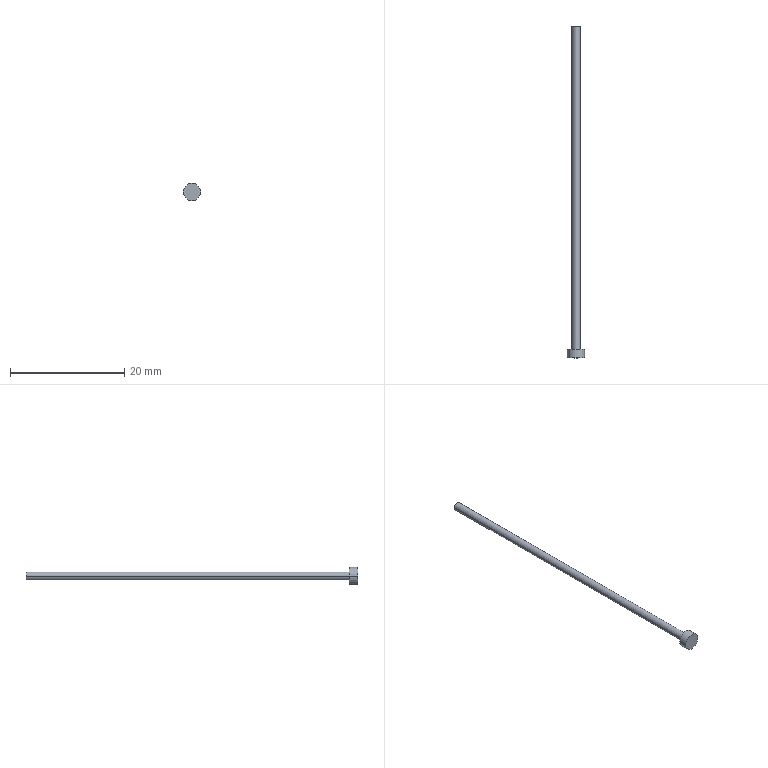Part | STEP file | ejector | 1 solid | 7 faces | box 3 x 58.08 x 3 mm | volume 97.701 mm3 | cylinder 4 | plane 3 | commonest cylinder face diameters 1.4 x2 3 x2
STEP:
#1=CARTESIAN_POINT('',(0.,0.,0.));
#2=DIRECTION('',(0.,0.,1.));
#3=DIRECTION('',(1.,0.,0.));
#4=AXIS2_PLACEMENT_3D('',#1,#2,#3);
#5=CARTESIAN_POINT('',(-0.7,1.5,0.));
#6=VERTEX_POINT('',#5);
#7=CARTESIAN_POINT('',(0.7,1.5,0.));
#8=VERTEX_POINT('',#7);
#9=CARTESIAN_POINT('',(0.,1.5,0.));
#10=DIRECTION('',(0.,1.,0.));
#11=DIRECTION('',(-1.,0.,0.));
#12=AXIS2_PLACEMENT_3D('',#9,#10,#11);
#13=CIRCLE('',#12,0.7);
#14=CARTESIAN_POINT('',(0.,58.08,0.));
#15=DIRECTION('',(0.,1.,0.));
#16=DIRECTION('',(-1.,0.,0.));
#17=AXIS2_PLACEMENT_3D('',#14,#15,#16);
#18=CYLINDRICAL_SURFACE('',#17,0.7);
#19=CARTESIAN_POINT('',(0.,-56.58));
#20=DIRECTION('',(1.,0.));
#21=VECTOR('',#20,1.);
#22=LINE('',#19,#21);
#23=(GEOMETRIC_REPRESENTATION_CONTEXT(2)PARAMETRIC_REPRESENTATION_CONTEXT()REPRESENTATION_CONTEXT('',''));
#24=DEFINITIONAL_REPRESENTATION('',(#22),#23);
#25=PCURVE('',#18,#24);
#26=CARTESIAN_POINT('',(-1.5,1.5,0.));
#27=DIRECTION('',(0.,1.,0.));
#28=DIRECTION('',(-1.,0.,0.));
#29=AXIS2_PLACEMENT_3D('',#26,#27,#28);
#30=PLANE('',#29);
#31=CARTESIAN_POINT('',(-1.5,0.));
#32=DIRECTION('',(1.,0.));
#33=AXIS2_PLACEMENT_2D('',#31,#32);
#34=CIRCLE('',#33,0.7);
#35=(GEOMETRIC_REPRESENTATION_CONTEXT(2)PARAMETRIC_REPRESENTATION_CONTEXT()REPRESENTATION_CONTEXT('',''));
#36=DEFINITIONAL_REPRESENTATION('',(#34),#35);
#37=PCURVE('',#30,#36);
#38=SURFACE_CURVE('',#13,(#25,#37),.PCURVE_S1.);
#39=EDGE_CURVE('',#6,#8,#38,.T.);
#40=ORIENTED_EDGE('',*,*,#39,.T.);
#41=CARTESIAN_POINT('',(0.7,58.08,0.));
#42=VERTEX_POINT('',#41);
#43=CARTESIAN_POINT('',(0.7,58.08,0.));
#44=DIRECTION('',(0.,1.,0.));
#45=VECTOR('',#44,1.);
#46=LINE('',#43,#45);
#47=CARTESIAN_POINT('',(3.142,0.));
#48=DIRECTION('',(0.,1.));
#49=VECTOR('',#48,1.);
#50=LINE('',#47,#49);
#51=(GEOMETRIC_REPRESENTATION_CONTEXT(2)PARAMETRIC_REPRESENTATION_CONTEXT()REPRESENTATION_CONTEXT('',''));
#52=DEFINITIONAL_REPRESENTATION('',(#50),#51);
#53=PCURVE('',#18,#52);
#54=CARTESIAN_POINT('',(0.,58.08,0.));
#55=DIRECTION('',(0.,1.,0.));
#56=DIRECTION('',(-1.,0.,0.));
#57=AXIS2_PLACEMENT_3D('',#54,#55,#56);
#58=CYLINDRICAL_SURFACE('',#57,0.7);
#59=CARTESIAN_POINT('',(3.142,0.));
#60=DIRECTION('',(0.,1.));
#61=VECTOR('',#60,1.);
#62=LINE('',#59,#61);
#63=(GEOMETRIC_REPRESENTATION_CONTEXT(2)PARAMETRIC_REPRESENTATION_CONTEXT()REPRESENTATION_CONTEXT('',''));
#64=DEFINITIONAL_REPRESENTATION('',(#62),#63);
#65=PCURVE('',#58,#64);
#66=SURFACE_CURVE('',#46,(#53,#65),.PCURVE_S1.);
#67=EDGE_CURVE('',#8,#42,#66,.T.);
#68=ORIENTED_EDGE('',*,*,#67,.T.);
#69=CARTESIAN_POINT('',(-0.7,58.08,0.));
#70=VERTEX_POINT('',#69);
#71=CARTESIAN_POINT('',(0.,58.08,0.));
#72=DIRECTION('',(0.,1.,0.));
#73=DIRECTION('',(-1.,0.,0.));
#74=AXIS2_PLACEMENT_3D('',#71,#72,#73);
#75=CIRCLE('',#74,0.7);
#76=CARTESIAN_POINT('',(0.,0.));
#77=DIRECTION('',(1.,0.));
#78=VECTOR('',#77,1.);
#79=LINE('',#76,#78);
#80=(GEOMETRIC_REPRESENTATION_CONTEXT(2)PARAMETRIC_REPRESENTATION_CONTEXT()REPRESENTATION_CONTEXT('',''));
#81=DEFINITIONAL_REPRESENTATION('',(#79),#80);
#82=PCURVE('',#18,#81);
#83=CARTESIAN_POINT('',(-0.7,58.08,0.));
#84=DIRECTION('',(0.,1.,0.));
#85=DIRECTION('',(-1.,0.,0.));
#86=AXIS2_PLACEMENT_3D('',#83,#84,#85);
#87=PLANE('',#86);
#88=CARTESIAN_POINT('',(-0.7,0.));
#89=DIRECTION('',(1.,0.));
#90=AXIS2_PLACEMENT_2D('',#88,#89);
#91=CIRCLE('',#90,0.7);
#92=(GEOMETRIC_REPRESENTATION_CONTEXT(2)PARAMETRIC_REPRESENTATION_CONTEXT()REPRESENTATION_CONTEXT('',''));
#93=DEFINITIONAL_REPRESENTATION('',(#91),#92);
#94=PCURVE('',#87,#93);
#95=SURFACE_CURVE('',#75,(#82,#94),.PCURVE_S1.);
#96=EDGE_CURVE('',#70,#42,#95,.T.);
#97=ORIENTED_EDGE('',*,*,#96,.F.);
#98=CARTESIAN_POINT('',(-0.7,58.08,0.));
#99=DIRECTION('',(0.,1.,0.));
#100=VECTOR('',#99,1.);
#101=LINE('',#98,#100);
#102=CARTESIAN_POINT('',(0.,0.));
#103=DIRECTION('',(0.,1.));
#104=VECTOR('',#103,1.);
#105=LINE('',#102,#104);
#106=(GEOMETRIC_REPRESENTATION_CONTEXT(2)PARAMETRIC_REPRESENTATION_CONTEXT()REPRESENTATION_CONTEXT('',''));
#107=DEFINITIONAL_REPRESENTATION('',(#105),#106);
#108=PCURVE('',#18,#107);
#109=CARTESIAN_POINT('',(6.283,0.));
#110=DIRECTION('',(0.,1.));
#111=VECTOR('',#110,1.);
#112=LINE('',#109,#111);
#113=(GEOMETRIC_REPRESENTATION_CONTEXT(2)PARAMETRIC_REPRESENTATION_CONTEXT()REPRESENTATION_CONTEXT('',''));
#114=DEFINITIONAL_REPRESENTATION('',(#112),#113);
#115=PCURVE('',#58,#114);
#116=SURFACE_CURVE('',#101,(#108,#115),.PCURVE_S1.);
#117=EDGE_CURVE('',#6,#70,#116,.T.);
#118=ORIENTED_EDGE('',*,*,#117,.F.);
#119=EDGE_LOOP('',(#40,#68,#97,#118));
#120=FACE_BOUND('',#119,.T.);
#121=ADVANCED_FACE('',(#120),#18,.T.);
#122=CARTESIAN_POINT('',(-1.5,0.,0.));
#123=VERTEX_POINT('',#122);
#124=CARTESIAN_POINT('',(1.5,0.,0.));
#125=VERTEX_POINT('',#124);
#126=CARTESIAN_POINT('',(0.,0.,0.));
#127=DIRECTION('',(0.,1.,0.));
#128=DIRECTION('',(-1.,0.,0.));
#129=AXIS2_PLACEMENT_3D('',#126,#127,#128);
#130=CIRCLE('',#129,1.5);
#131=CARTESIAN_POINT('',(0.,58.08,0.));
#132=DIRECTION('',(0.,1.,0.));
#133=DIRECTION('',(-1.,0.,0.));
#134=AXIS2_PLACEMENT_3D('',#131,#132,#133);
#135=CYLINDRICAL_SURFACE('',#134,1.5);
#136=CARTESIAN_POINT('',(0.,-58.08));
#137=DIRECTION('',(1.,0.));
#138=VECTOR('',#137,1.);
#139=LINE('',#136,#138);
#140=(GEOMETRIC_REPRESENTATION_CONTEXT(2)PARAMETRIC_REPRESENTATION_CONTEXT()REPRESENTATION_CONTEXT('',''));
#141=DEFINITIONAL_REPRESENTATION('',(#139),#140);
#142=PCURVE('',#135,#141);
#143=CARTESIAN_POINT('',(0.,0.,0.));
#144=DIRECTION('',(0.,-1.,0.));
#145=DIRECTION('',(1.,0.,0.));
#146=AXIS2_PLACEMENT_3D('',#143,#144,#145);
#147=PLANE('',#146);
#148=CARTESIAN_POINT('',(-1.5,0.));
#149=CARTESIAN_POINT('',(-1.5,2.598));
#150=CARTESIAN_POINT('',(0.75,1.299));
#151=CARTESIAN_POINT('',(3.,0.));
#152=CARTESIAN_POINT('',(0.75,-1.299));
#153=CARTESIAN_POINT('',(-1.5,-2.598));
#154=CARTESIAN_POINT('',(-1.5,0.));
#155=(BOUNDED_CURVE()B_SPLINE_CURVE(2,(#148,#149,#150,#151,#152,#153,#154),.UNSPECIFIED.,.T.,.F.)B_SPLINE_CURVE_WITH_KNOTS((1,2,2,2,2,1),(-2.094,0.,2.094,4.189,6.283,8.378),.UNSPECIFIED.)CURVE()GEOMETRIC_REPRESENTATION_ITEM()RATIONAL_B_SPLINE_CURVE((1.,0.5,1.,0.5,1.,0.5,1.))REPRESENTATION_ITEM(''));
#156=(GEOMETRIC_REPRESENTATION_CONTEXT(2)PARAMETRIC_REPRESENTATION_CONTEXT()REPRESENTATION_CONTEXT('',''));
#157=DEFINITIONAL_REPRESENTATION('',(#155),#156);
#158=PCURVE('',#147,#157);
#159=SURFACE_CURVE('',#130,(#142,#158),.PCURVE_S1.);
#160=EDGE_CURVE('',#123,#125,#159,.T.);
#161=ORIENTED_EDGE('',*,*,#160,.T.);
#162=CARTESIAN_POINT('',(1.5,1.5,0.));
#163=VERTEX_POINT('',#162);
#164=CARTESIAN_POINT('',(1.5,58.08,0.));
#165=DIRECTION('',(0.,1.,0.));
#166=VECTOR('',#165,1.);
#167=LINE('',#164,#166);
#168=CARTESIAN_POINT('',(3.142,0.));
#169=DIRECTION('',(0.,1.));
#170=VECTOR('',#169,1.);
#171=LINE('',#168,#170);
#172=(GEOMETRIC_REPRESENTATION_CONTEXT(2)PARAMETRIC_REPRESENTATION_CONTEXT()REPRESENTATION_CONTEXT('',''));
#173=DEFINITIONAL_REPRESENTATION('',(#171),#172);
#174=PCURVE('',#135,#173);
#175=CARTESIAN_POINT('',(0.,58.08,0.));
#176=DIRECTION('',(0.,1.,0.));
#177=DIRECTION('',(-1.,0.,0.));
#178=AXIS2_PLACEMENT_3D('',#175,#176,#177);
#179=CYLINDRICAL_SURFACE('',#178,1.5);
#180=CARTESIAN_POINT('',(3.142,0.));
#181=DIRECTION('',(0.,1.));
#182=VECTOR('',#181,1.);
#183=LINE('',#180,#182);
#184=(GEOMETRIC_REPRESENTATION_CONTEXT(2)PARAMETRIC_REPRESENTATION_CONTEXT()REPRESENTATION_CONTEXT('',''));
#185=DEFINITIONAL_REPRESENTATION('',(#183),#184);
#186=PCURVE('',#179,#185);
#187=SURFACE_CURVE('',#167,(#174,#186),.PCURVE_S1.);
#188=EDGE_CURVE('',#125,#163,#187,.T.);
#189=ORIENTED_EDGE('',*,*,#188,.T.);
#190=CARTESIAN_POINT('',(-1.5,1.5,0.));
#191=VERTEX_POINT('',#190);
#192=CARTESIAN_POINT('',(0.,1.5,0.));
#193=DIRECTION('',(0.,1.,0.));
#194=DIRECTION('',(-1.,0.,0.));
#195=AXIS2_PLACEMENT_3D('',#192,#193,#194);
#196=CIRCLE('',#195,1.5);
#197=CARTESIAN_POINT('',(0.,-56.58));
#198=DIRECTION('',(1.,0.));
#199=VECTOR('',#198,1.);
#200=LINE('',#197,#199);
#201=(GEOMETRIC_REPRESENTATION_CONTEXT(2)PARAMETRIC_REPRESENTATION_CONTEXT()REPRESENTATION_CONTEXT('',''));
#202=DEFINITIONAL_REPRESENTATION('',(#200),#201);
#203=PCURVE('',#135,#202);
#204=CARTESIAN_POINT('',(-1.5,0.));
#205=DIRECTION('',(1.,0.));
#206=AXIS2_PLACEMENT_2D('',#204,#205);
#207=CIRCLE('',#206,1.5);
#208=(GEOMETRIC_REPRESENTATION_CONTEXT(2)PARAMETRIC_REPRESENTATION_CONTEXT()REPRESENTATION_CONTEXT('',''));
#209=DEFINITIONAL_REPRESENTATION('',(#207),#208);
#210=PCURVE('',#30,#209);
#211=SURFACE_CURVE('',#196,(#203,#210),.PCURVE_S1.);
#212=EDGE_CURVE('',#191,#163,#211,.T.);
#213=ORIENTED_EDGE('',*,*,#212,.F.);
#214=CARTESIAN_POINT('',(-1.5,58.08,0.));
#215=DIRECTION('',(0.,1.,0.));
#216=VECTOR('',#215,1.);
#217=LINE('',#214,#216);
#218=CARTESIAN_POINT('',(0.,0.));
#219=DIRECTION('',(0.,1.));
#220=VECTOR('',#219,1.);
#221=LINE('',#218,#220);
#222=(GEOMETRIC_REPRESENTATION_CONTEXT(2)PARAMETRIC_REPRESENTATION_CONTEXT()REPRESENTATION_CONTEXT('',''));
#223=DEFINITIONAL_REPRESENTATION('',(#221),#222);
#224=PCURVE('',#135,#223);
#225=CARTESIAN_POINT('',(6.283,0.));
#226=DIRECTION('',(0.,1.));
#227=VECTOR('',#226,1.);
#228=LINE('',#225,#227);
#229=(GEOMETRIC_REPRESENTATION_CONTEXT(2)PARAMETRIC_REPRESENTATION_CONTEXT()REPRESENTATION_CONTEXT('',''));
#230=DEFINITIONAL_REPRESENTATION('',(#228),#229);
#231=PCURVE('',#179,#230);
#232=SURFACE_CURVE('',#217,(#224,#231),.PCURVE_S1.);
#233=EDGE_CURVE('',#123,#191,#232,.T.);
#234=ORIENTED_EDGE('',*,*,#233,.F.);
#235=EDGE_LOOP('',(#161,#189,#213,#234));
#236=FACE_BOUND('',#235,.T.);
#237=ADVANCED_FACE('',(#236),#135,.T.);
#238=ORIENTED_EDGE('',*,*,#160,.F.);
#239=CARTESIAN_POINT('',(0.,0.,0.));
#240=DIRECTION('',(0.,1.,0.));
#241=DIRECTION('',(-1.,0.,0.));
#242=AXIS2_PLACEMENT_3D('',#239,#240,#241);
#243=CIRCLE('',#242,1.5);
#244=CARTESIAN_POINT('',(-1.5,0.));
#245=CARTESIAN_POINT('',(-1.5,2.598));
#246=CARTESIAN_POINT('',(0.75,1.299));
#247=CARTESIAN_POINT('',(3.,0.));
#248=CARTESIAN_POINT('',(0.75,-1.299));
#249=CARTESIAN_POINT('',(-1.5,-2.598));
#250=CARTESIAN_POINT('',(-1.5,0.));
#251=(BOUNDED_CURVE()B_SPLINE_CURVE(2,(#244,#245,#246,#247,#248,#249,#250),.UNSPECIFIED.,.T.,.F.)B_SPLINE_CURVE_WITH_KNOTS((1,2,2,2,2,1),(-2.094,0.,2.094,4.189,6.283,8.378),.UNSPECIFIED.)CURVE()GEOMETRIC_REPRESENTATION_ITEM()RATIONAL_B_SPLINE_CURVE((1.,0.5,1.,0.5,1.,0.5,1.))REPRESENTATION_ITEM(''));
#252=(GEOMETRIC_REPRESENTATION_CONTEXT(2)PARAMETRIC_REPRESENTATION_CONTEXT()REPRESENTATION_CONTEXT('',''));
#253=DEFINITIONAL_REPRESENTATION('',(#251),#252);
#254=PCURVE('',#147,#253);
#255=CARTESIAN_POINT('',(0.,-58.08));
#256=DIRECTION('',(1.,0.));
#257=VECTOR('',#256,1.);
#258=LINE('',#255,#257);
#259=(GEOMETRIC_REPRESENTATION_CONTEXT(2)PARAMETRIC_REPRESENTATION_CONTEXT()REPRESENTATION_CONTEXT('',''));
#260=DEFINITIONAL_REPRESENTATION('',(#258),#259);
#261=PCURVE('',#179,#260);
#262=SURFACE_CURVE('',#243,(#254,#261),.PCURVE_S1.);
#263=EDGE_CURVE('',#125,#123,#262,.T.);
#264=ORIENTED_EDGE('',*,*,#263,.F.);
#265=EDGE_LOOP('',(#238,#264));
#266=FACE_BOUND('',#265,.T.);
#267=ADVANCED_FACE('',(#266),#147,.T.);
#268=ORIENTED_EDGE('',*,*,#188,.F.);
#269=ORIENTED_EDGE('',*,*,#263,.T.);
#270=ORIENTED_EDGE('',*,*,#233,.T.);
#271=CARTESIAN_POINT('',(0.,1.5,0.));
#272=DIRECTION('',(0.,1.,0.));
#273=DIRECTION('',(-1.,0.,0.));
#274=AXIS2_PLACEMENT_3D('',#271,#272,#273);
#275=CIRCLE('',#274,1.5);
#276=CARTESIAN_POINT('',(0.,-56.58));
#277=DIRECTION('',(1.,0.));
#278=VECTOR('',#277,1.);
#279=LINE('',#276,#278);
#280=(GEOMETRIC_REPRESENTATION_CONTEXT(2)PARAMETRIC_REPRESENTATION_CONTEXT()REPRESENTATION_CONTEXT('',''));
#281=DEFINITIONAL_REPRESENTATION('',(#279),#280);
#282=PCURVE('',#179,#281);
#283=CARTESIAN_POINT('',(-1.5,0.));
#284=DIRECTION('',(1.,0.));
#285=AXIS2_PLACEMENT_2D('',#283,#284);
#286=CIRCLE('',#285,1.5);
#287=(GEOMETRIC_REPRESENTATION_CONTEXT(2)PARAMETRIC_REPRESENTATION_CONTEXT()REPRESENTATION_CONTEXT('',''));
#288=DEFINITIONAL_REPRESENTATION('',(#286),#287);
#289=PCURVE('',#30,#288);
#290=SURFACE_CURVE('',#275,(#282,#289),.PCURVE_S1.);
#291=EDGE_CURVE('',#163,#191,#290,.T.);
#292=ORIENTED_EDGE('',*,*,#291,.F.);
#293=EDGE_LOOP('',(#268,#269,#270,#292));
#294=FACE_BOUND('',#293,.T.);
#295=ADVANCED_FACE('',(#294),#179,.T.);
#296=ORIENTED_EDGE('',*,*,#212,.T.);
#297=ORIENTED_EDGE('',*,*,#291,.T.);
#298=EDGE_LOOP('',(#296,#297));
#299=FACE_BOUND('',#298,.T.);
#300=ORIENTED_EDGE('',*,*,#39,.F.);
#301=CARTESIAN_POINT('',(0.,1.5,0.));
#302=DIRECTION('',(0.,1.,0.));
#303=DIRECTION('',(-1.,0.,0.));
#304=AXIS2_PLACEMENT_3D('',#301,#302,#303);
#305=CIRCLE('',#304,0.7);
#306=CARTESIAN_POINT('',(-1.5,0.));
#307=DIRECTION('',(1.,0.));
#308=AXIS2_PLACEMENT_2D('',#306,#307);
#309=CIRCLE('',#308,0.7);
#310=(GEOMETRIC_REPRESENTATION_CONTEXT(2)PARAMETRIC_REPRESENTATION_CONTEXT()REPRESENTATION_CONTEXT('',''));
#311=DEFINITIONAL_REPRESENTATION('',(#309),#310);
#312=PCURVE('',#30,#311);
#313=CARTESIAN_POINT('',(0.,-56.58));
#314=DIRECTION('',(1.,0.));
#315=VECTOR('',#314,1.);
#316=LINE('',#313,#315);
#317=(GEOMETRIC_REPRESENTATION_CONTEXT(2)PARAMETRIC_REPRESENTATION_CONTEXT()REPRESENTATION_CONTEXT('',''));
#318=DEFINITIONAL_REPRESENTATION('',(#316),#317);
#319=PCURVE('',#58,#318);
#320=SURFACE_CURVE('',#305,(#312,#319),.PCURVE_S1.);
#321=EDGE_CURVE('',#8,#6,#320,.T.);
#322=ORIENTED_EDGE('',*,*,#321,.F.);
#323=EDGE_LOOP('',(#300,#322));
#324=FACE_BOUND('',#323,.T.);
#325=ADVANCED_FACE('',(#299,#324),#30,.T.);
#326=ORIENTED_EDGE('',*,*,#67,.F.);
#327=ORIENTED_EDGE('',*,*,#321,.T.);
#328=ORIENTED_EDGE('',*,*,#117,.T.);
#329=CARTESIAN_POINT('',(0.,58.08,0.));
#330=DIRECTION('',(0.,1.,0.));
#331=DIRECTION('',(-1.,0.,0.));
#332=AXIS2_PLACEMENT_3D('',#329,#330,#331);
#333=CIRCLE('',#332,0.7);
#334=CARTESIAN_POINT('',(0.,0.));
#335=DIRECTION('',(1.,0.));
#336=VECTOR('',#335,1.);
#337=LINE('',#334,#336);
#338=(GEOMETRIC_REPRESENTATION_CONTEXT(2)PARAMETRIC_REPRESENTATION_CONTEXT()REPRESENTATION_CONTEXT('',''));
#339=DEFINITIONAL_REPRESENTATION('',(#337),#338);
#340=PCURVE('',#58,#339);
#341=CARTESIAN_POINT('',(-0.7,0.));
#342=DIRECTION('',(1.,0.));
#343=AXIS2_PLACEMENT_2D('',#341,#342);
#344=CIRCLE('',#343,0.7);
#345=(GEOMETRIC_REPRESENTATION_CONTEXT(2)PARAMETRIC_REPRESENTATION_CONTEXT()REPRESENTATION_CONTEXT('',''));
#346=DEFINITIONAL_REPRESENTATION('',(#344),#345);
#347=PCURVE('',#87,#346);
#348=SURFACE_CURVE('',#333,(#340,#347),.PCURVE_S1.);
#349=EDGE_CURVE('',#42,#70,#348,.T.);
#350=ORIENTED_EDGE('',*,*,#349,.F.);
#351=EDGE_LOOP('',(#326,#327,#328,#350));
#352=FACE_BOUND('',#351,.T.);
#353=ADVANCED_FACE('',(#352),#58,.T.);
#354=ORIENTED_EDGE('',*,*,#96,.T.);
#355=ORIENTED_EDGE('',*,*,#349,.T.);
#356=EDGE_LOOP('',(#354,#355));
#357=FACE_BOUND('',#356,.T.);
#358=ADVANCED_FACE('',(#357),#87,.T.);
#359=CLOSED_SHELL('',(#121,#237,#267,#295,#325,#353,#358));
#360=MANIFOLD_SOLID_BREP('',#359);
#361=(LENGTH_UNIT()NAMED_UNIT(*)SI_UNIT(.MILLI.,.METRE.));
#362=UNCERTAINTY_MEASURE_WITH_UNIT(LENGTH_MEASURE(0.0000001),#361,'','');
#363=(NAMED_UNIT(*)PLANE_ANGLE_UNIT()SI_UNIT($,.RADIAN.));
#364=(NAMED_UNIT(*)SI_UNIT($,.STERADIAN.)SOLID_ANGLE_UNIT());
#365=(GEOMETRIC_REPRESENTATION_CONTEXT(3)GLOBAL_UNCERTAINTY_ASSIGNED_CONTEXT((#362))GLOBAL_UNIT_ASSIGNED_CONTEXT((#361,#363,#364))REPRESENTATION_CONTEXT('',''));
#366=ADVANCED_BREP_SHAPE_REPRESENTATION('',(#4,#360),#365);